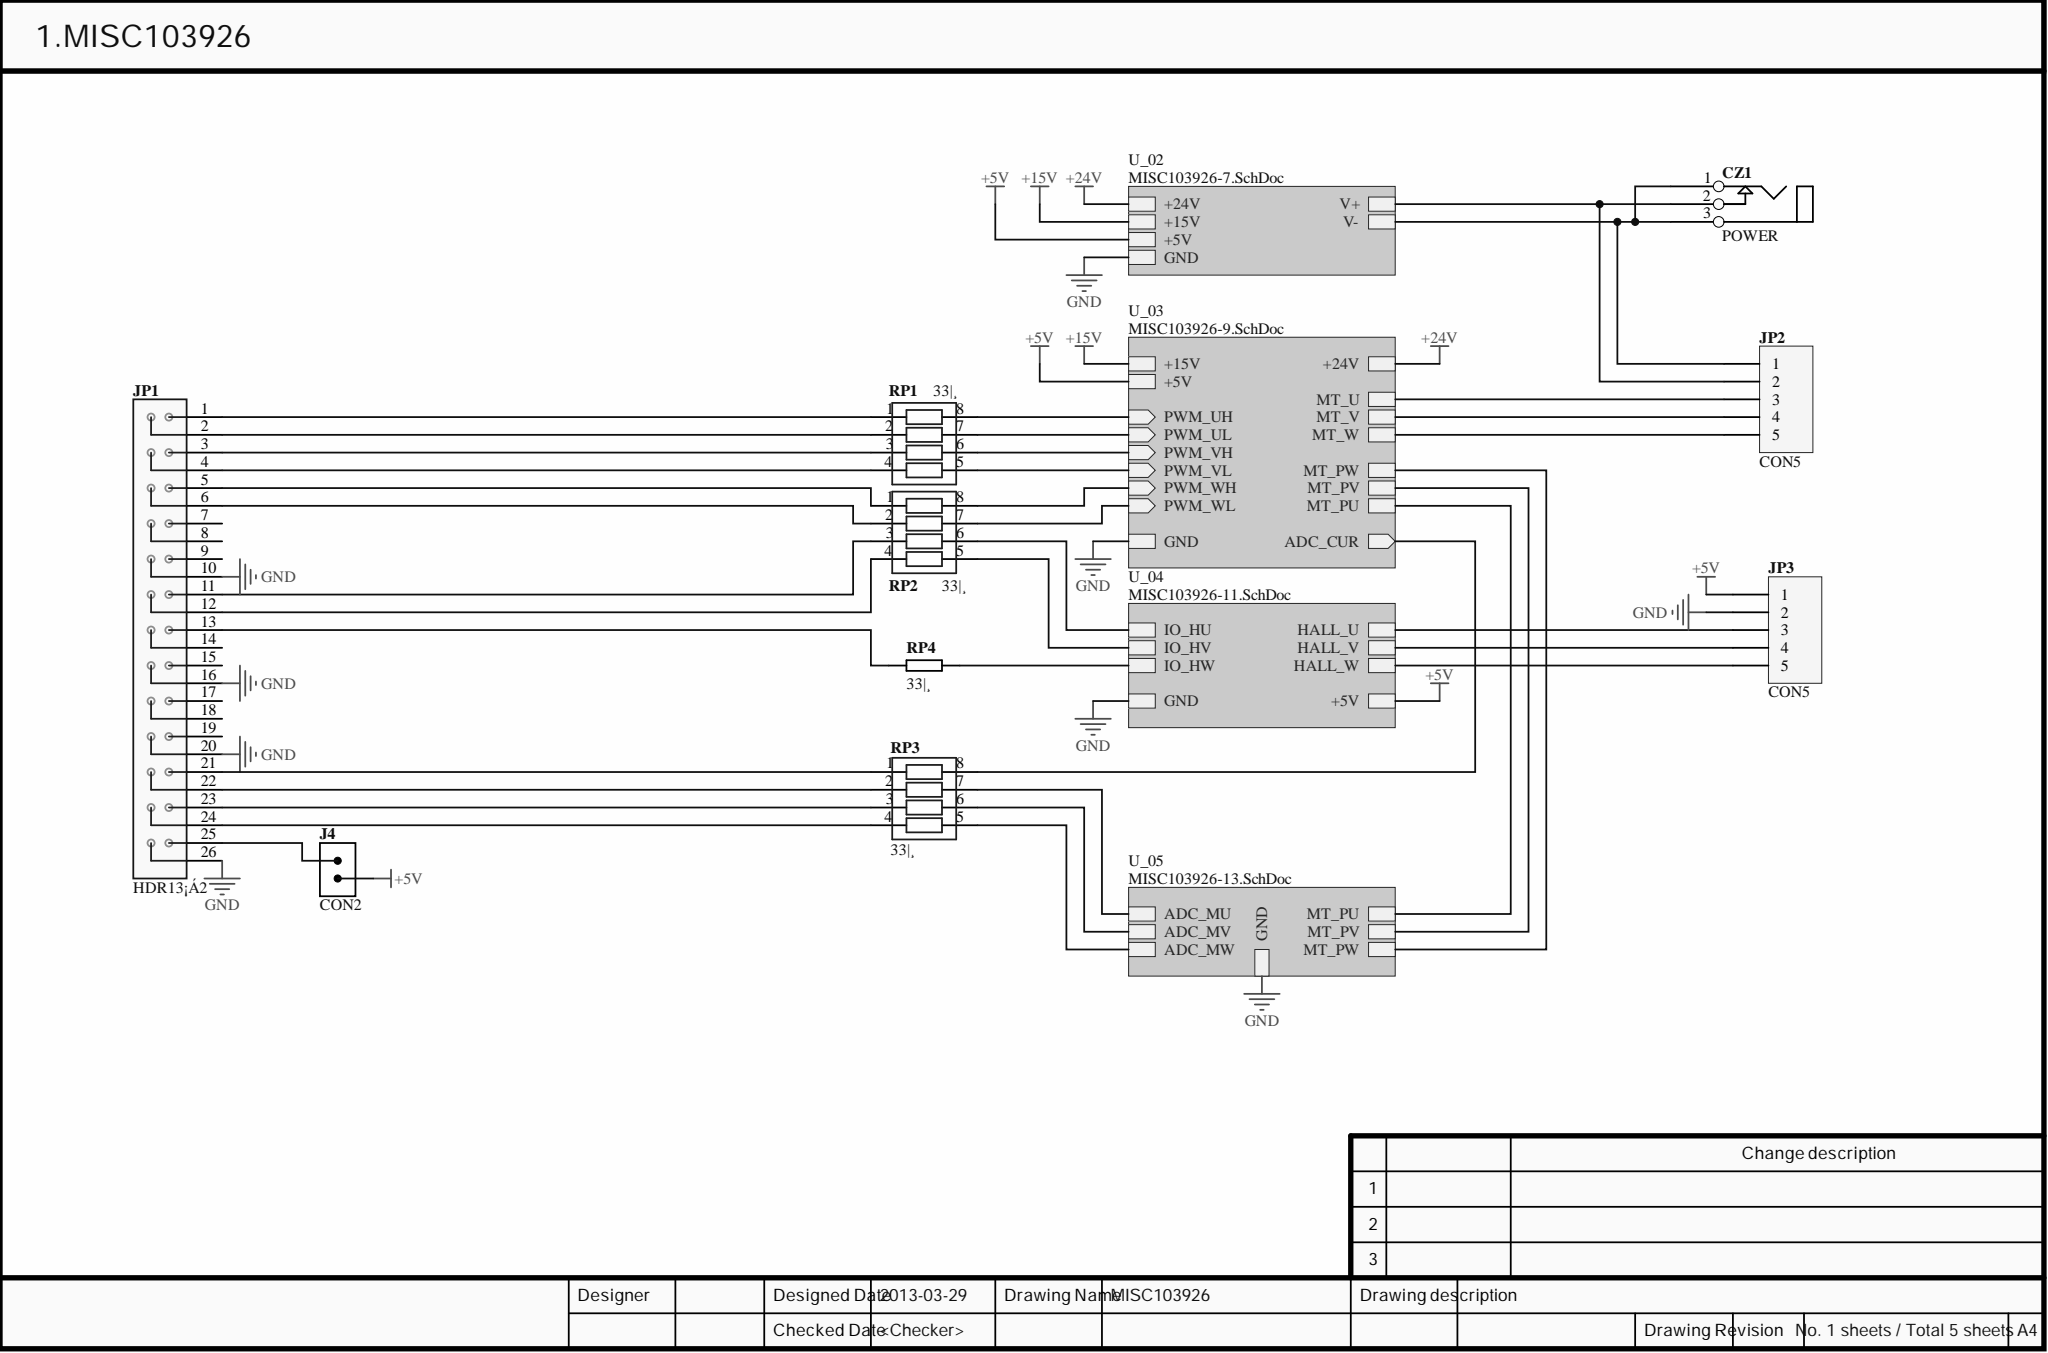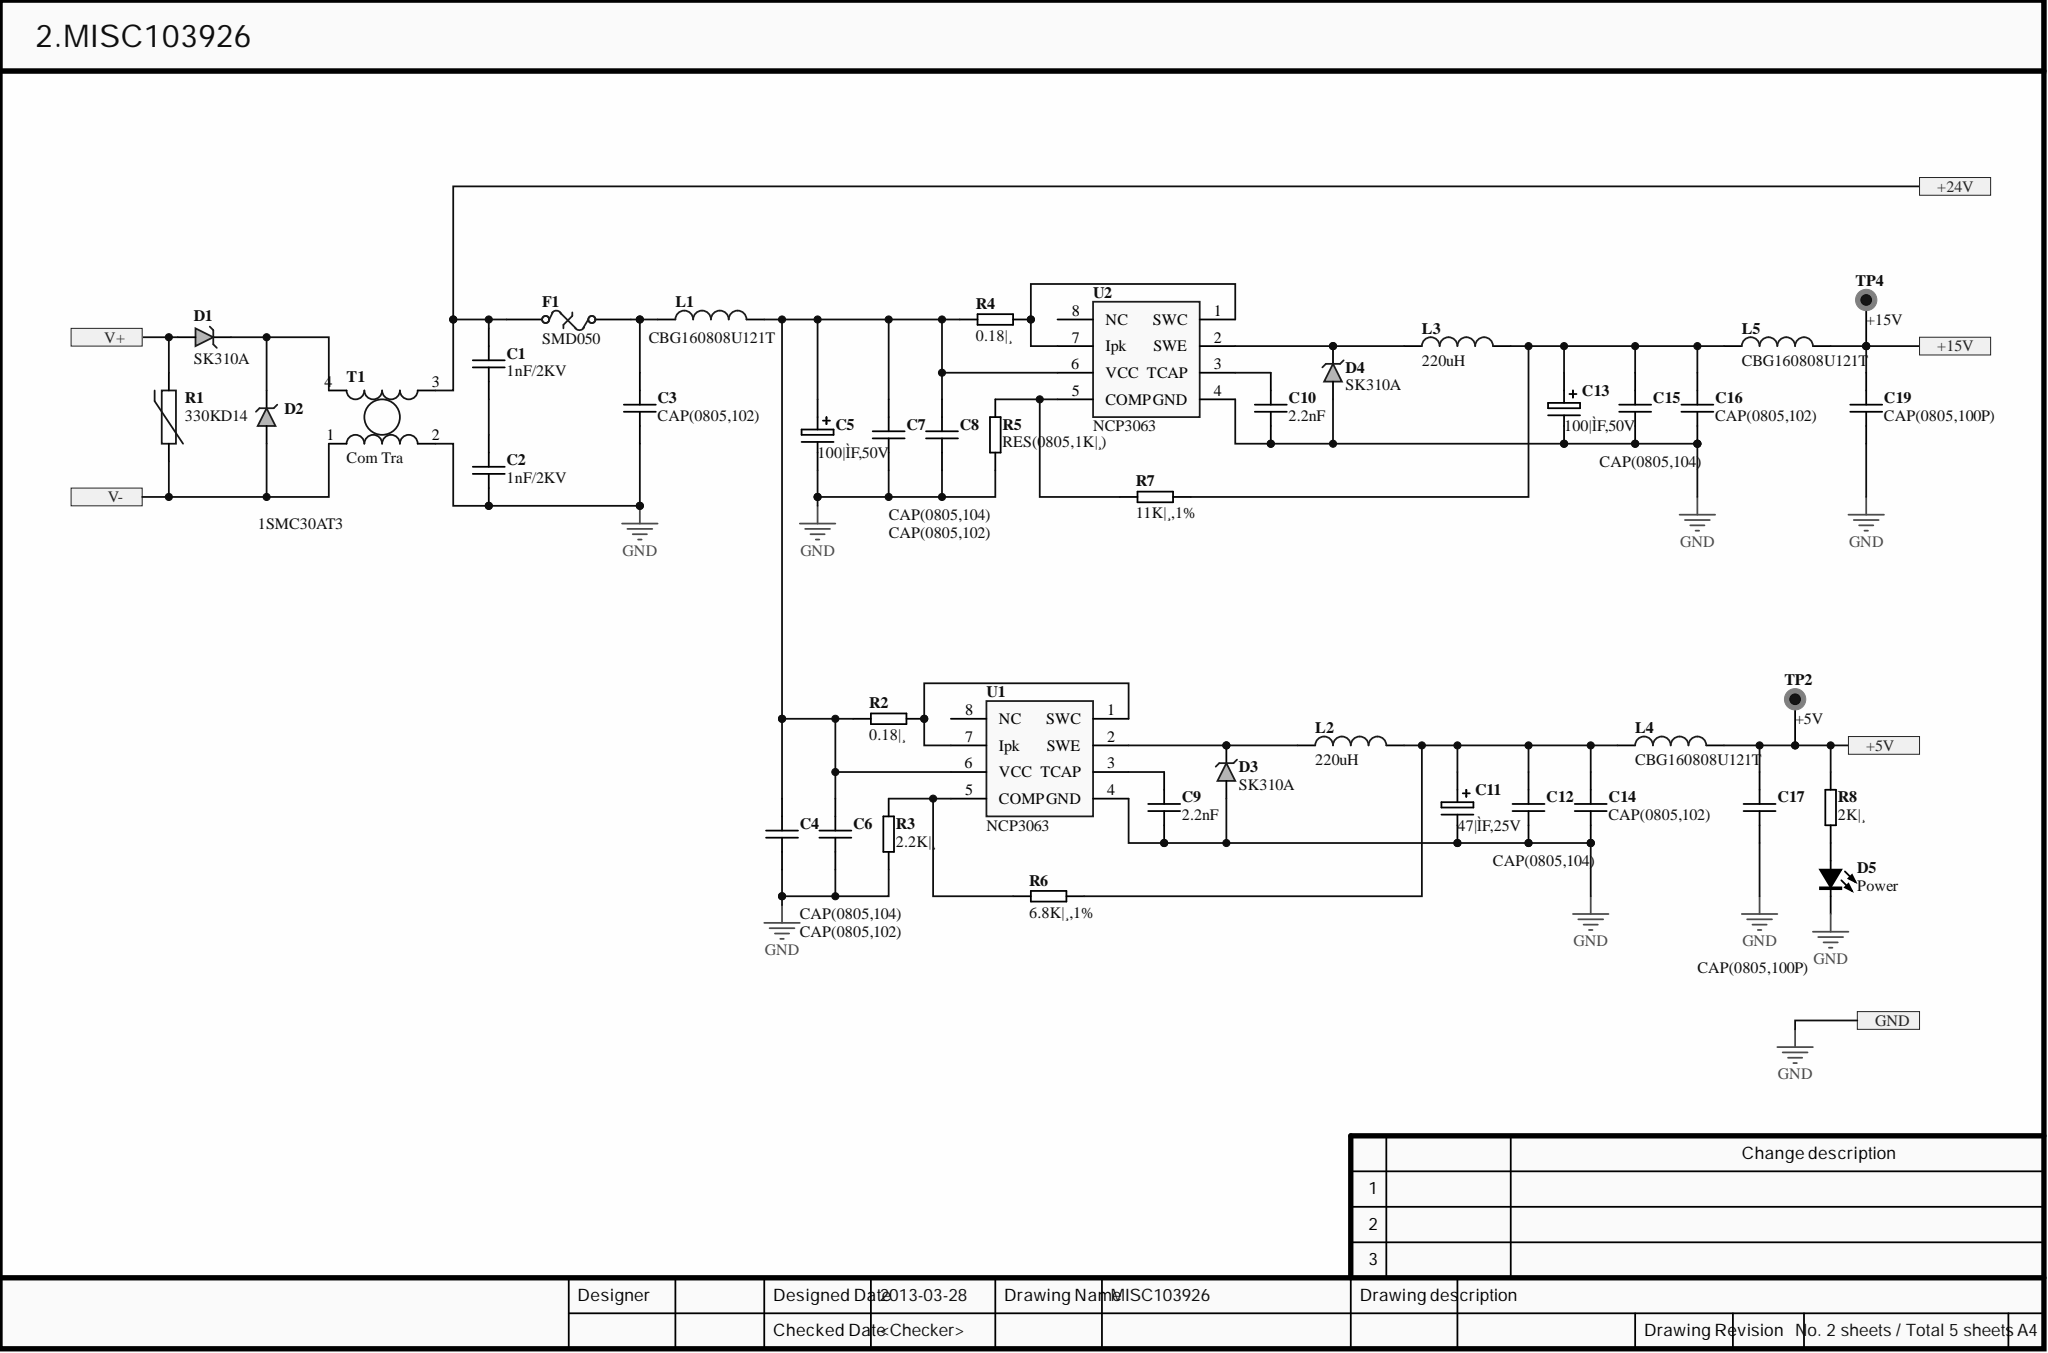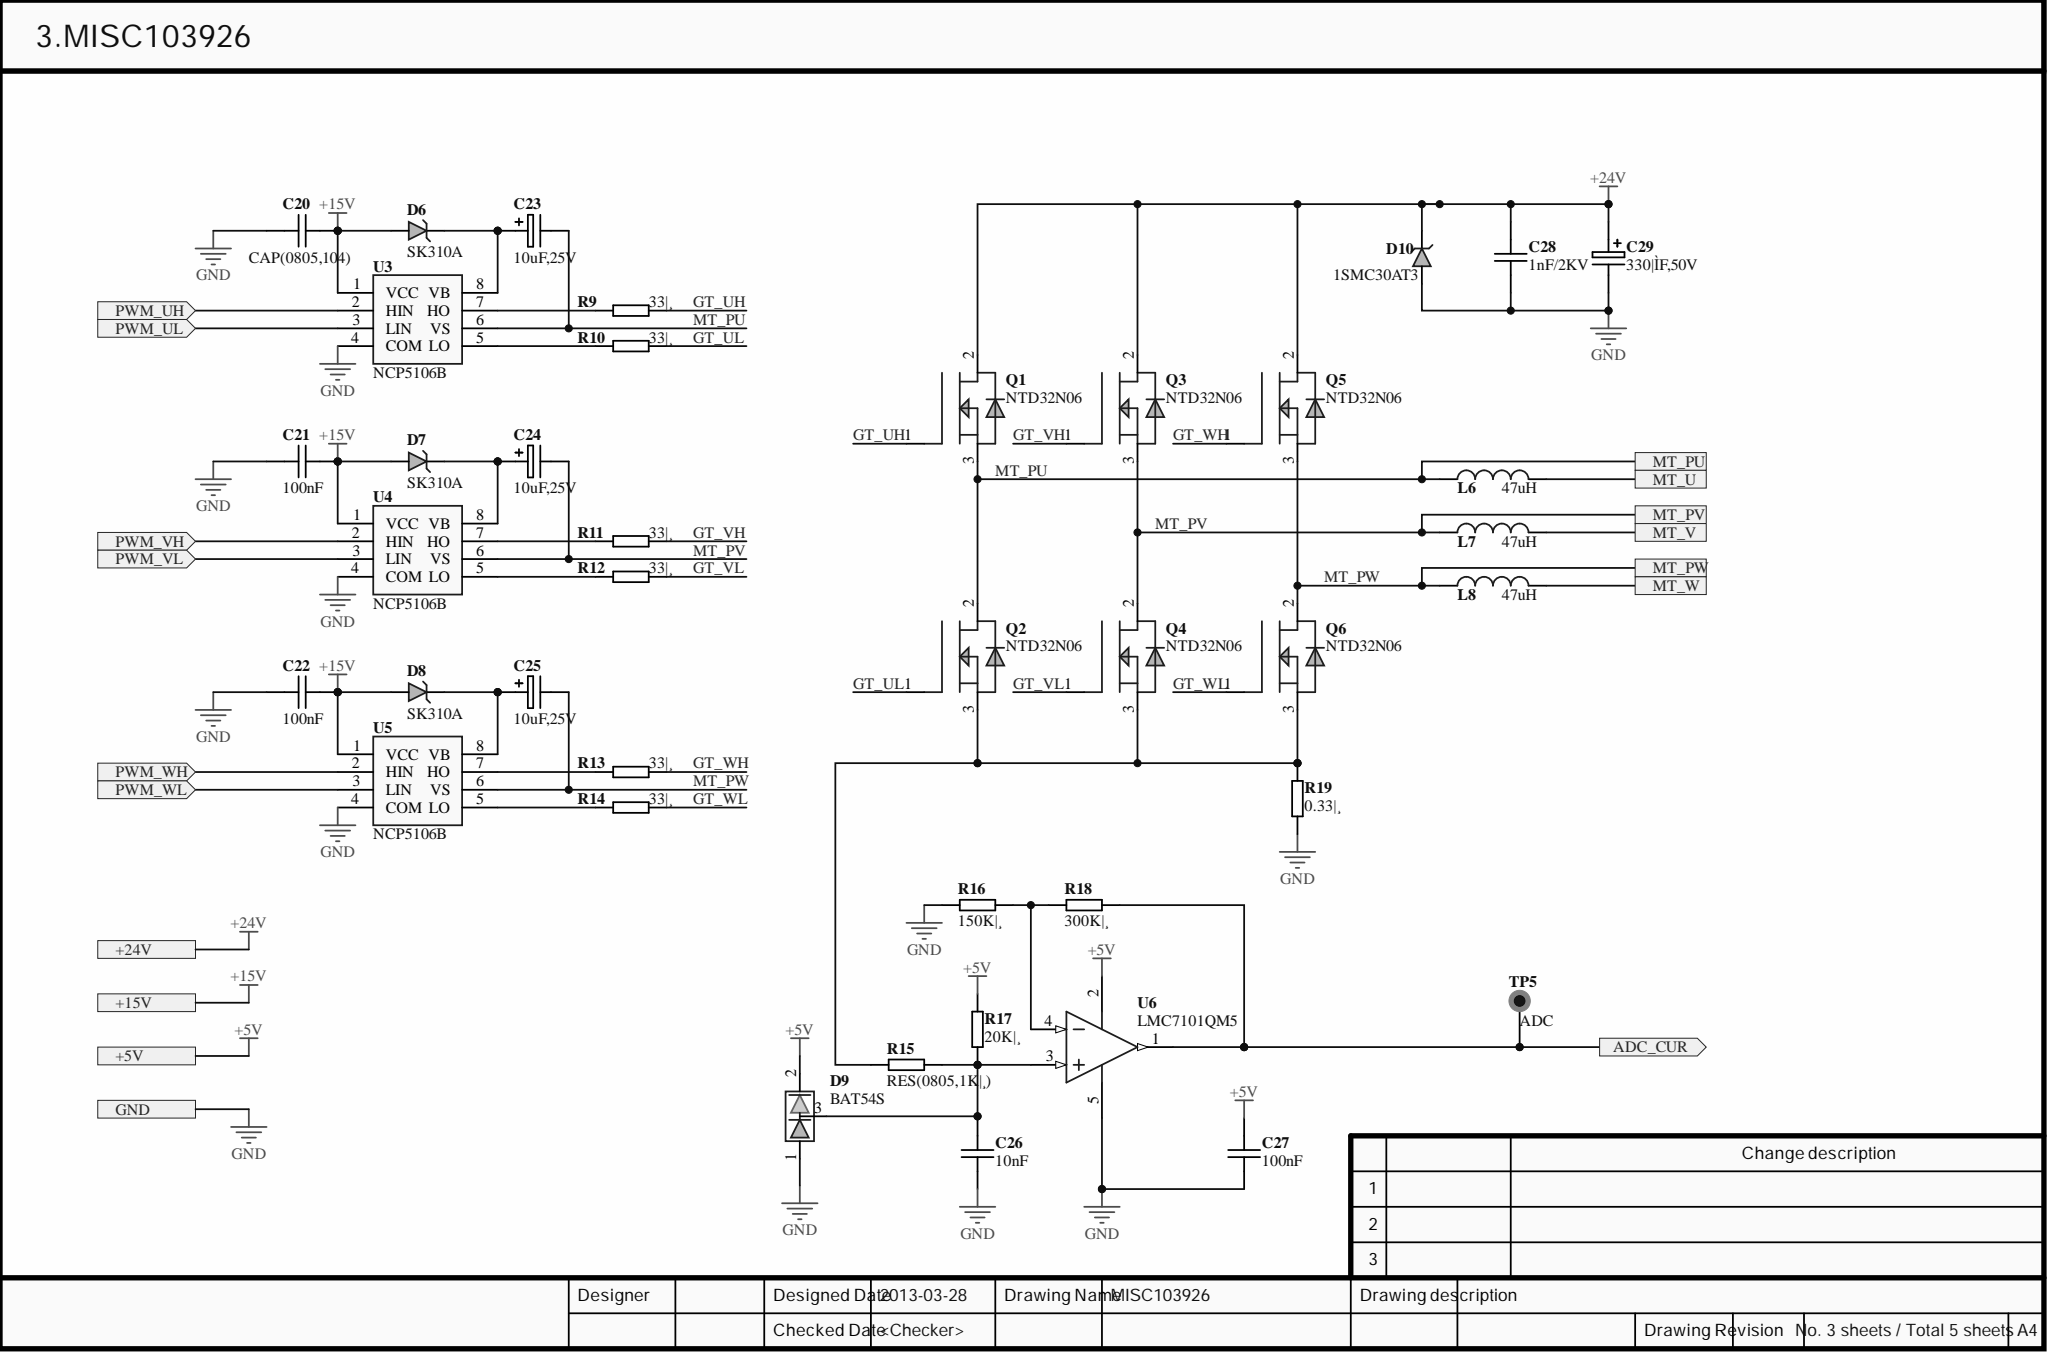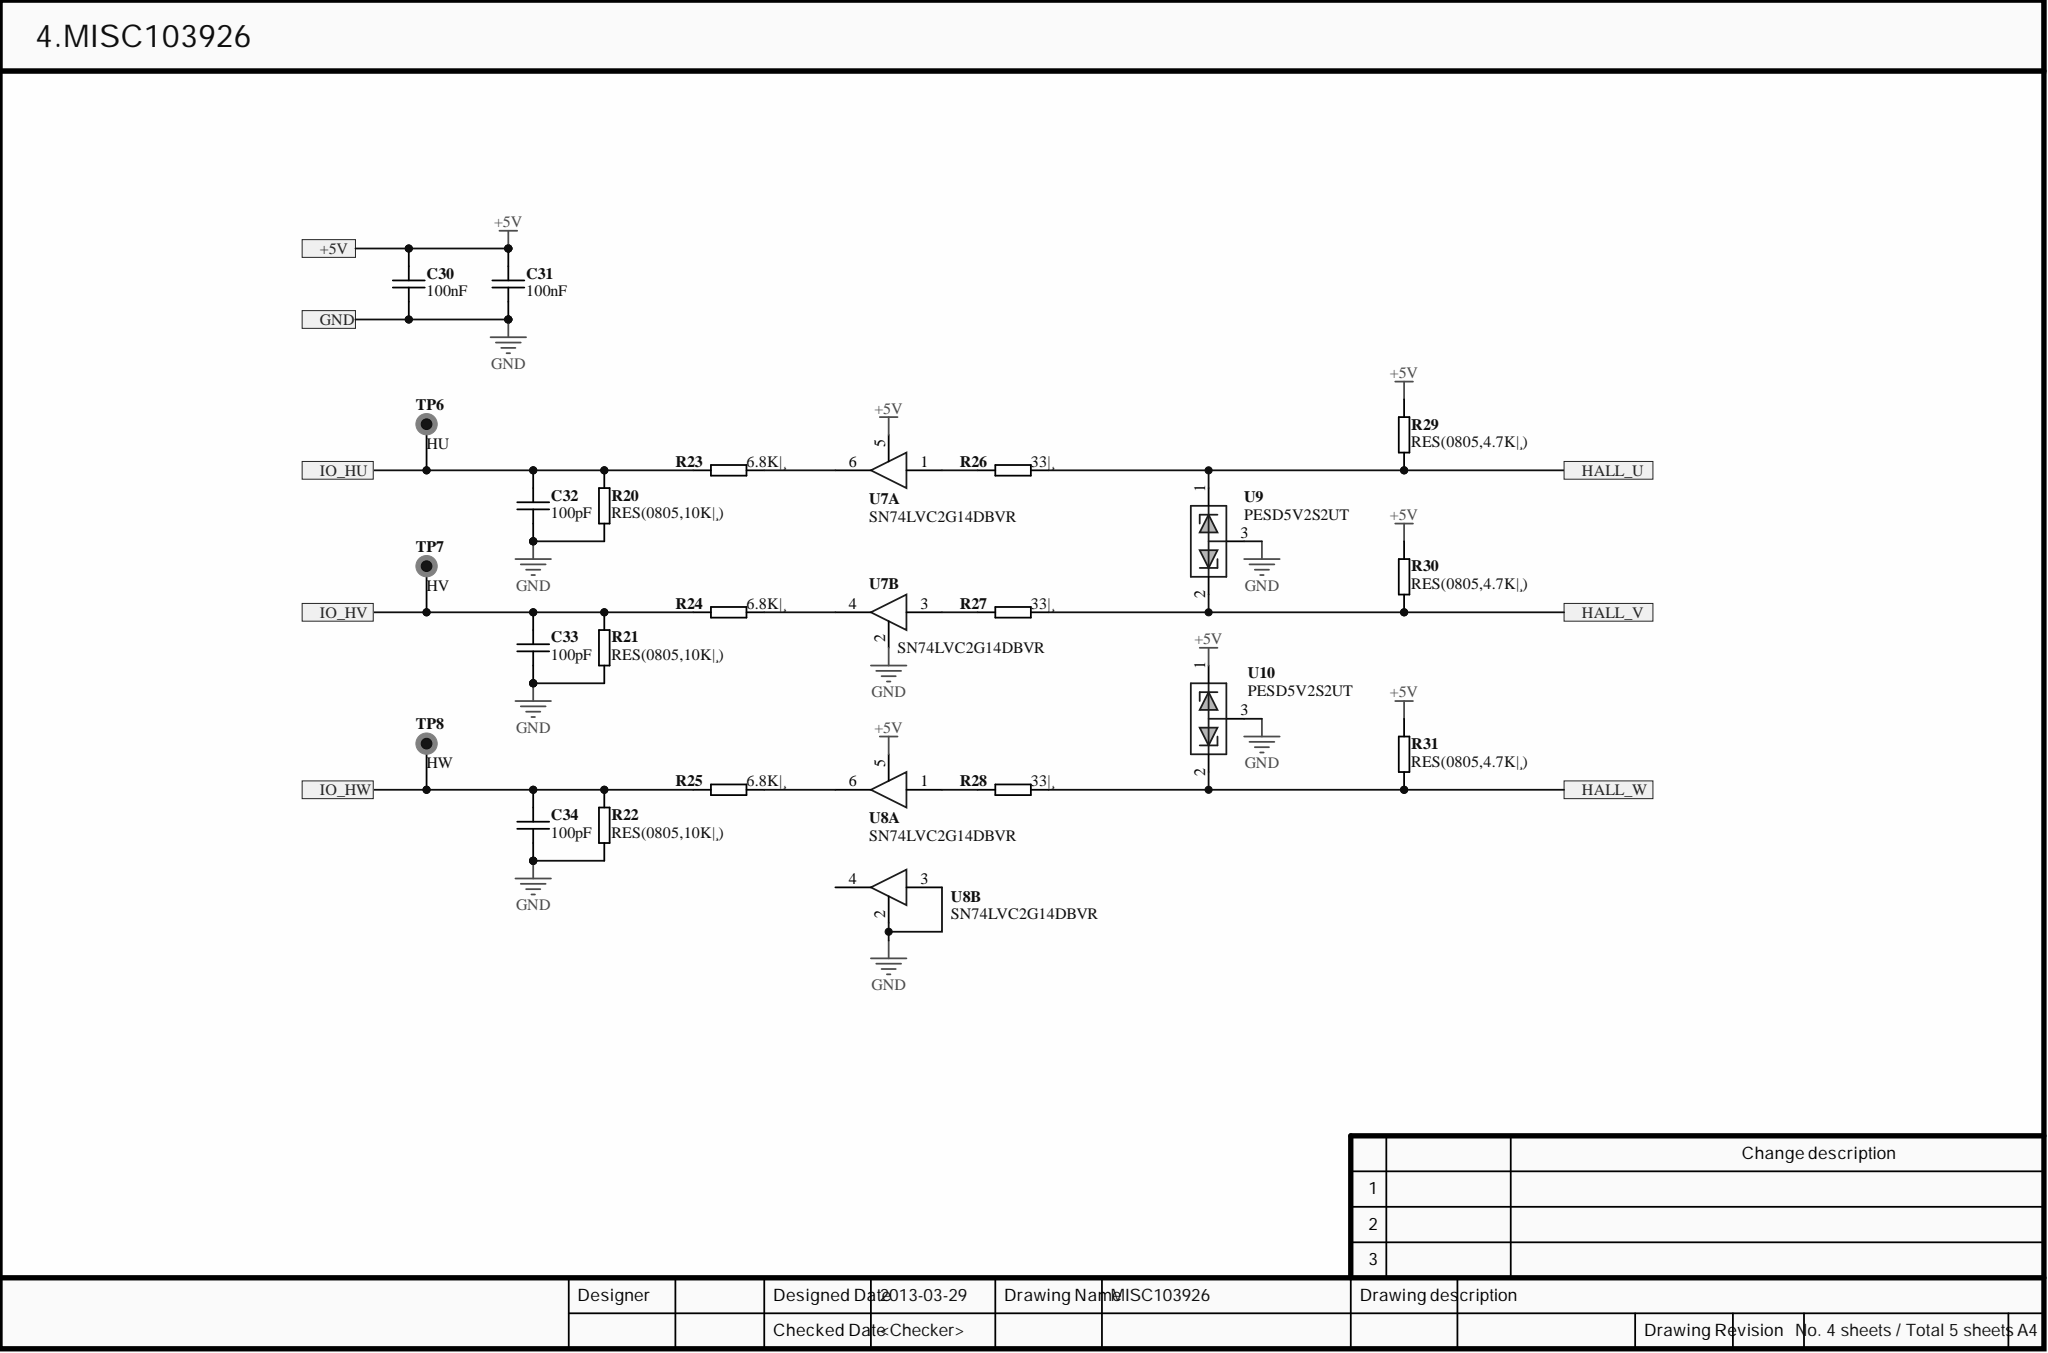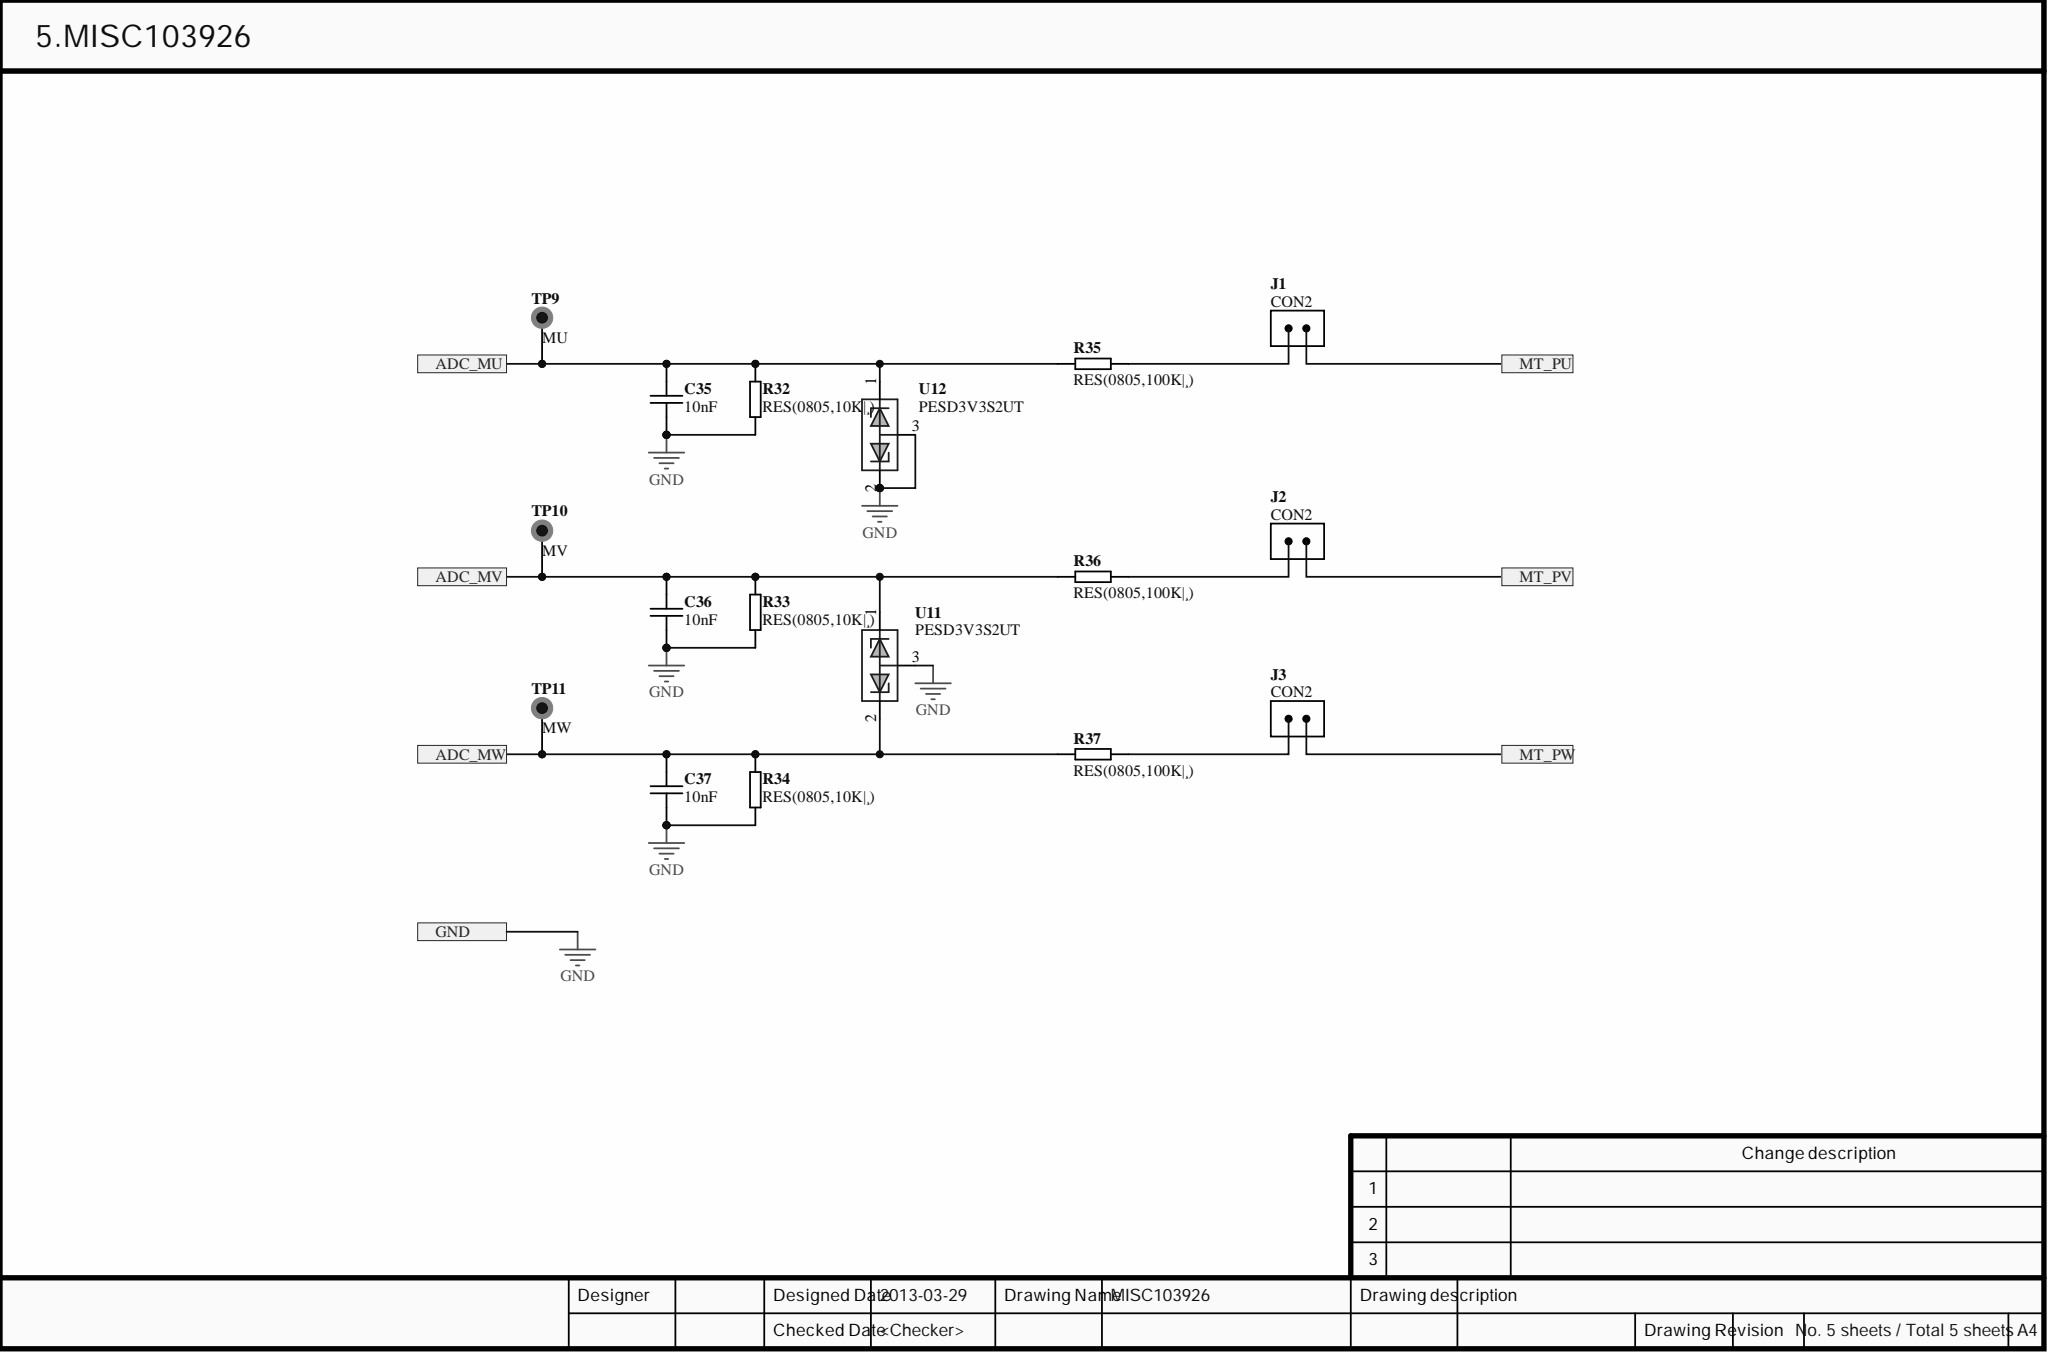Circuit board | Altium Designer | 132 parts | 84 nets
Bill of materials:
Comment,Description,Designator,Footprint,LibRef,Quantity
"1nF/2KV","1.02.03.0003","C1, C2, C28","1206C","CAP(1206,102,2KV)","3"
"CAP(0805,102)","1.02.02.0028","C3, C6, C8, C14, C16","0805C","CAP(0805,102)","5"
"CAP(0805,104)","1.02.02.0038","C4, C7, C12, C15, C20","0805C","CAP(0805,104)","5"
"100|ÌF,50V","[NoValue], SMD capacitor","C5, C13","CAP-D","CAP(电解,100UF,16V,Ф6.3×5)","2"
"2.2nF","2.2nF, 24 to 5v power use, 2.2nF, 24 to 15 power use","C9, C10","0805C","CAP(0805,103)","2"
"47|ÌF,25V","","C11","CAP-D","CAP(电解,100UF,16V,Ф6.3×5)","1"
"CAP(0805,100P)","1.02.02.0019","C17, C19","0805C","CAP(0805,100P)","2"
"100nF","1.02.02.0038","C21, C22, C27, C30, C31","0805C","CAP(0805,104)","5"
"10uF,25V","SMD capacitor, [NoValue]","C23, C24, C25","CAP-C","CAP(电解,10UF,25V,Ф4×7)","3"
"10nF","1.02.02.0032","C26, C35, C36, C37","0805C","CAP(0805,103)","4"
"330|ÌF,50V","Electrolytic capacitor","C29","电解电容","CAP(电解,100UF,16V,Ф6.3×5)","1"
"100pF","1.02.02.0019","C32, C33, C34","0805C","CAP(0805,100P)","3"
"POWER","","CZ1","POWER-AC","电源座(3.5-2.1,黑色)","1"
"SK310A","SK310A","D1, D3, D4, D6, D7, D8","DO-214AC","","6"
"1SMC30AT3","TVS diode","D2, D10","1SMC17AT","","2"
"Power","1.04.05.0001","D5","0805D","LED(0805,红色)","1"
"BAT54S","Diode","D9","SOT-23","","1"
"SMD050","Resettable fuse","F1","1812DT","Fuse Thermal","1"
"CON2","","J1, J2, J3, J4","SIP-2","CN-2","4"
"HDR13¡Á2","HDR13¡Á2","JP1","IDC-26","","1"
"CON5","CON5","JP2","CON-5-5.0","MHDR1X5","1"
"CON5","Header, 5-Pin","JP3","CON-5-3.81","MHDR1X5","1"
"CBG160808U121T","Inductor","L1, L4, L5","0603C","Inductor","3"
"220uH","Inductor","L2, L3","L-7.5S","Inductor","2"
"47uH","Inductor","L6, L7, L8","L-7.5S","Inductor","3"
"NTD32N06","MOSFET","Q1, Q2, Q3, Q4, Q5, Q6","DPAK-3","","6"
"330KD14","Varistor","R1","AX-.3/.6","","1"
"0.18|¸","","R2, R4","2512","RES(0805,0|¸)","2"
"2.2K|¸","1.01.02.0044","R3","0805R","RES(0805,1K|¸)","1"
"RES(0805,1K|¸)","1.01.02.0044","R5, R15","0805R","RES(0805,1K|¸)","2"
"6.8K|¸,1%","","R6","0805R","RES(0805,1K|¸)","1"
"11K|¸,1%","","R7","0805R","RES(0805,1K|¸)","1"
"2K|¸","","R8","0805R","RES(0805,2.2K|¸)","1"
"33|¸","1.01.02.0017","R9, R10, R11, R12, R13, R14, R26, R27, R28, RP4","0805R","RES(0805,33|¸)","10"
"150K|¸","","R16","0805R","RES(0805,300K|¸)","1"
"20K|¸","","R17","0805R","RES(0805,300K|¸)","1"
"300K|¸","1.01.02.0097","R18","0805R","RES(0805,300K|¸)","1"
"0.33|¸","1.01.02.0001","R19","2512","RES(0805,0|¸)","1"
"RES(0805,10K|¸)","1.01.02.0067","R20, R21, R22, R32, R33, R34","0805R","RES(0805,10K|¸)","6"
"6.8K|¸","","R23, R24, R25","0805R","RES(0805,33|¸)","3"
"RES(0805,4.7K|¸)","1.01.02.0059","R29, R30, R31","0805R","RES(0805,4.7K|¸)","3"
"RES(0805,100K|¸)","1.01.02.0092","R35, R36, R37","0805R","RES(0805,100K|¸)","3"
"33|¸","Resistor array","RP1, RP2, RP3","PZ-4-0.8B","","3"
"Com Tra","Choke coil","T1","L-2-XIAO","","1"
"+5V","1.10.03.0153","TP2","PAD(60)","圆孔针(1P)","1"
"+15V","1.10.03.0153","TP4","PAD(60)","圆孔针(1P)","1"
"ADC","1.10.03.0153","TP5","PAD(60)","圆孔针(1P)","1"
"HU","1.10.03.0153","TP6","PAD(60)","圆孔针(1P)","1"
"HV","1.10.03.0153","TP7","PAD(60)","圆孔针(1P)","1"
"HW","1.10.03.0153","TP8","PAD(60)","圆孔针(1P)","1"
"MU","1.10.03.0153","TP9","PAD(60)","圆孔针(1P)","1"
"MV","1.10.03.0153","TP10","PAD(60)","圆孔针(1P)","1"
"MW","1.10.03.0153","TP11","PAD(60)","圆孔针(1P)","1"
"NCP3063","IC","U1, U2","SO-8","","2"
"NCP5106B","IC","U3, U4, U5","SO-8","","3"
"LMC7101QM5","Tiny Low Power Operational Amplifier with Rail-to-Rail Input and Output","U6","MF05A_N","LMC7101QM5","1"
"SN74LVC2G14DBVR","IC","U7, U8","SOT-23-6","","2"
"PESD5V2S2UT","IC","U9, U10","SOT-23","","2"
"PESD3V3S2UT","IC","U11, U12","SOT-23","","2"
Netlist (Protel format):
[
C1
1206C
1nF/2KV



]
[
C2
1206C
1nF/2KV



]
[
C3
0805C
CAP(0805,102)



]
[
C4
0805C
CAP(0805,104)



]
[
C5
CAP-D
100|ÌF,50V



]
[
C6
0805C
CAP(0805,102)



]
[
C7
0805C
CAP(0805,104)



]
[
C8
0805C
CAP(0805,102)



]
[
C9
0805C
2.2nF



]
[
C10
0805C
2.2nF



]
[
C11
CAP-D
47|ÌF,25V



]
[
C12
0805C
CAP(0805,104)



]
[
C13
CAP-D
100|ÌF,50V



]
[
C14
0805C
CAP(0805,102)



]
[
C15
0805C
CAP(0805,104)



]
[
C16
0805C
CAP(0805,102)



]
[
C17
0805C
CAP(0805,100P)



]
[
C19
0805C
CAP(0805,100P)



]
[
C20
0805C
CAP(0805,104)



]
[
C21
0805C
100nF



]
[
C22
0805C
100nF



]
[
C23
CAP-C
10uF,25V



]
[
C24
CAP-C
10uF,25V



]
[
C25
CAP-C
10uF,25V



]
[
C26
0805C
10nF



]
[
C27
0805C
100nF



]
[
C28
1206C
1nF/2KV



]
[
C29
电解电容
330|ÌF,50V



]
[
C30
0805C
100nF



]
[
C31
0805C
100nF



]
[
C32
0805C
100pF



]
[
C33
0805C
100pF



]
[
C34
0805C
100pF



]
[
C35
0805C
10nF



]
[
C36
0805C
10nF



]
[
C37
0805C
10nF



]
[
CZ1
POWER-AC
POWER



]
[
D1
DO-214AC
SK310A



]
[
D2
1SMC17AT
1SMC30AT3



]
[
D3
DO-214AC
SK310A



]
[
D4
DO-214AC
SK310A



]
[
D5
0805D
Power



]
[
D6
DO-214AC
SK310A



]
[
D7
DO-214AC
SK310A



]
[
D8
DO-214AC
SK310A



]
[
D9
SOT-23
BAT54S



]
[
D10
1SMC17AT
1SMC30AT3



]
[
F1
1812DT
SMD050



]
[
J1
SIP-2
CON2



]
[
J2
SIP-2
CON2



]
[
J3
SIP-2
CON2



]
[
J4
SIP-2
CON2



]
[
JP1
IDC-26
HDR13¡Á2



]
[
JP2
CON-5-5.0
CON5



]
[
JP3
CON-5-3.81
CON5



]
[
L1
0603C
CBG160808U121T



]
[
L2
L-7.5S
220uH



]
[
L3
L-7.5S
220uH



]
[
L4
0603C
CBG160808U121T



]
[
L5
0603C
CBG160808U121T



]
[
L6
L-7.5S
47uH



]
[
L7
L-7.5S
47uH



]
[
L8
L-7.5S
47uH



]
[
Q1
DPAK-3
NTD32N06



]
[
Q2
DPAK-3
NTD32N06



]
[
Q3
DPAK-3
NTD32N06



]
[
Q4
DPAK-3
NTD32N06



]
[
Q5
DPAK-3
NTD32N06



]
[
Q6
DPAK-3
NTD32N06



]
[
R1
AX-.3/.6
330KD14



]
[
R2
2512
0.18|¸



]
[
R3
0805R
2.2K|¸



]
[
R4
2512
0.18|¸



]
[
R5
0805R
RES(0805,1K|¸)



]
[
R6
0805R
6.8K|¸,1%



]
[
R7
0805R
11K|¸,1%



]
[
R8
0805R
2K|¸



]
[
R9
0805R
33|¸



]
[
R10
0805R
33|¸



]
[
R11
0805R
33|¸



]
[
R12
0805R
33|¸



]
[
R13
0805R
33|¸



]
[
R14
0805R
33|¸



]
[
R15
0805R
RES(0805,1K|¸)



]
[
R16
0805R
150K|¸



]
[
R17
0805R
20K|¸



]
[
R18
0805R
300K|¸



]
[
R19
2512
0.33|¸



]
[
R20
0805R
RES(0805,10K|¸)



]
[
R21
0805R
RES(0805,10K|¸)



]
[
R22
0805R
RES(0805,10K|¸)



]
[
R23
0805R
6.8K|¸



]
[
R24
0805R
6.8K|¸



]
[
R25
0805R
6.8K|¸



]
[
R26
0805R
33|¸



]
[
R27
0805R
33|¸



]
[
R28
0805R
33|¸



]
[
R29
0805R
RES(0805,4.7K|¸)



]
[
R30
0805R
RES(0805,4.7K|¸)



]
[
R31
0805R
RES(0805,4.7K|¸)



]
[
R32
0805R
RES(0805,10K|¸)



]
[
R33
0805R
RES(0805,10K|¸)



]
[
R34
0805R
RES(0805,10K|¸)



]
[
R35
0805R
RES(0805,100K|¸)



]
[
R36
0805R
RES(0805,100K|¸)



]
[
R37
0805R
RES(0805,100K|¸)



]
[
RP1
PZ-4-0.8B
33|¸



]
[
RP2
PZ-4-0.8B
33|¸



]
[
RP3
PZ-4-0.8B
33|¸



]
[
RP4
0805R
33|¸



]
[
T1
L-2-XIAO
Com Tra



]
[
TP2
PAD(60)
+5V



]
[
TP4
PAD(60)
+15V



]
[
TP5
PAD(60)
ADC



]
[
TP6
PAD(60)
HU



]
[
TP7
PAD(60)
HV



]
[
TP8
PAD(60)
HW



]
[
TP9
PAD(60)
MU



]
[
TP10
PAD(60)
MV



]
[
TP11
PAD(60)
MW



]
[
U1
SO-8
NCP3063



]
[
U2
SO-8
NCP3063



]
[
U3
SO-8
NCP5106B



]
[
U4
SO-8
NCP5106B



]
[
U5
SO-8
NCP5106B



]
[
U6
MF05A_N
LMC7101QM5



]
[
U7
SOT-23-6
SN74LVC2G14DBVR



]
[
U8
SOT-23-6
SN74LVC2G14DBVR



]
[
U9
SOT-23
PESD5V2S2UT



]
[
U10
SOT-23
PESD5V2S2UT



]
[
U11
SOT-23
PESD3V3S2UT



]
[
U12
SOT-23
PESD3V3S2UT



]
(
NetRP2_8
RP2-8
U5-2
)
(
NetRP2_7
RP2-7
U5-3
)
(
NetRP1_8
RP1-8
U3-2
)
(
NetRP1_7
RP1-7
U3-3
)
(
NetRP1_6
RP1-6
U4-2
)
(
NetRP1_5
RP1-5
U4-3
)
(
NetR28_1
R28-1
U8-1
)
(
NetR27_1
R27-1
U7-3
)
(
NetR26_1
R26-1
U7-1
)
(
NetR25_2
R25-2
U8-6
)
(
NetR24_2
R24-2
U7-4
)
(
NetR23_2
R23-2
U7-6
)
(
NetR18_1
R18-1
RP3-8
TP5-1
U6-1
)
(
NetR16_1
R16-1
R18-2
U6-4
)
(
NetR14_1
R14-1
U5-5
)
(
NetR13_1
R13-1
U5-7
)
(
NetR12_1
R12-1
U4-5
)
(
NetR11_1
R11-1
U4-7
)
(
NetR10_1
R10-1
U3-5
)
(
NetR9_1
R9-1
U3-7
)
(
NetR5_1
R5-1
R7-1
U2-5
)
(
NetR4_2
R4-2
U2-1
U2-7
)
(
NetR3_1
R3-1
R6-1
U1-5
)
(
NetR2_2
R2-2
U1-1
U1-7
)
(
NetQ2_3
Q2-3
Q4-3
Q6-3
R15-1
R19-2
)
(
NetJP3_5
JP3-5
R28-2
R31-2
U10-2
)
(
NetJP3_4
JP3-4
R27-2
R30-2
U9-2
)
(
NetJP3_3
JP3-3
R26-2
R29-2
U9-1
)
(
NetJP2_5
JP2-5
L8-2
)
(
NetJP2_4
JP2-4
L7-2
)
(
NetJP2_3
JP2-3
L6-2
)
(
NetJP1_24
JP1-24
RP3-4
)
(
NetJP1_23
JP1-23
RP3-3
)
(
NetJP1_22
JP1-22
RP3-2
)
(
NetJP1_21
JP1-21
RP3-1
)
(
NetJP1_13
JP1-13
RP4-1
)
(
NetJP1_12
JP1-12
RP2-4
)
(
NetJP1_11
JP1-11
RP2-3
)
(
NetJP1_6
JP1-6
RP2-2
)
(
NetJP1_5
JP1-5
RP2-1
)
(
NetJP1_4
JP1-4
RP1-4
)
(
NetJP1_3
JP1-3
RP1-3
)
(
NetJP1_2
JP1-2
RP1-2
)
(
NetJP1_1
JP1-1
RP1-1
)
(
NetJ4_2
J4-2
JP1-25
)
(
NetJ3_1
J3-1
R37-2
)
(
NetJ2_1
J2-1
R36-2
)
(
NetJ1_1
J1-1
R35-2
)
(
NetD5_1
D5-1
R8-2
)
(
NetD4_1
D4-1
L3-1
U2-2
)
(
NetD3_1
D3-1
L2-1
U1-2
)
(
NetD1_1
D1-1
D2-1
T1-4
)
(
NetCZ1_2
CZ1-2
D1-2
JP2-2
R1-1
)
(
NetCZ1_1
CZ1-1
CZ1-3
D2-2
JP2-1
R1-2
T1-1
)
(
NetC37_2
C37-2
R34-1
R37-1
RP3-5
TP11-1
U11-2
)
(
NetC36_2
C36-2
R33-1
R36-1
RP3-6
TP10-1
U11-1
)
(
NetC35_2
C35-2
R32-1
R35-1
RP3-7
TP9-1
U12-1
)
(
NetC34_1
C34-1
R22-1
R25-1
RP4-2
TP8-1
)
(
NetC33_1
C33-1
R21-1
R24-1
RP2-5
TP7-1
)
(
NetC32_1
C32-1
R20-1
R23-1
RP2-6
TP6-1
)
(
NetC26_2
C26-2
D9-3
R15-2
R17-2
U6-3
)
(
NetC25_1
C25-1
D8-1
U5-8
)
(
NetC24_1
C24-1
D7-1
U4-8
)
(
NetC23_1
C23-1
D6-1
U3-8
)
(
NetC13_1
C13-1
C15-1
C16-1
L3-2
L5-1
R7-2
)
(
NetC11_1
C11-1
C12-1
C14-1
L2-2
L4-1
R6-2
)
(
NetC10_1
C10-1
U2-3
)
(
NetC9_1
C9-1
U1-3
)
(
NetC4_1
C4-1
C5-1
C6-1
C7-1
C8-1
L1-2
R2-1
R4-1
U1-6
U2-6
)
(
NetC3_1
C3-1
F1-2
L1-1
)
(
NetC1_2
C1-2
C2-1
)
(
MT_PW
C25-2
J3-2
L8-1
Q5-3
Q6-2
U5-6
)
(
MT_PV
C24-2
J2-2
L7-1
Q3-3
Q4-2
U4-6
)
(
MT_PU
C23-2
J1-2
L6-1
Q1-3
Q2-2
U3-6
)
(
GT_WL
Q6-1
R14-2
)
(
GT_WH
Q5-1
R13-2
)
(
GT_VL
Q4-1
R12-2
)
(
GT_VH
Q3-1
R11-2
)
(
GT_UL
Q2-1
R10-2
)
(
GT_UH
Q1-1
R9-2
)
(
GND
C2-2
C3-2
C4-2
C5-2
C6-2
C7-2
C8-2
C9-2
C10-2
C11-2
C12-2
C13-2
C14-2
C15-2
C16-2
C17-2
C19-2
C20-1
C21-1
C22-1
C26-1
C27-1
C28-2
C29-2
C30-2
C31-1
C32-2
C33-2
C34-2
C35-1
C36-1
C37-1
D3-2
D4-2
D5-2
D9-1
D10-2
JP1-10
JP1-16
JP1-20
JP1-26
JP3-2
R3-2
R5-2
R16-2
R19-1
R20-2
R21-2
R22-2
R32-2
R33-2
R34-2
T1-2
U1-4
U2-4
U3-4
U4-4
U5-4
U6-5
U7-2
U8-2
U8-3
U9-3
U10-3
U11-3
U12-2
U12-3
)
(
+24V
C1-1
C28-1
C29-1
D10-1
F1-1
Q1-2
Q3-2
Q5-2
T1-3
)
(
+15V
C19-1
C20-2
C21-2
C22-2
D6-2
D7-2
D8-2
L5-2
TP4-1
U3-1
U4-1
U5-1
)
(
+5V
C17-1
C27-2
C30-1
C31-2
D9-2
J4-1
JP3-1
L4-2
R8-1
R17-1
R29-1
R30-1
R31-1
TP2-1
U6-2
U7-5
U8-5
U10-1
)